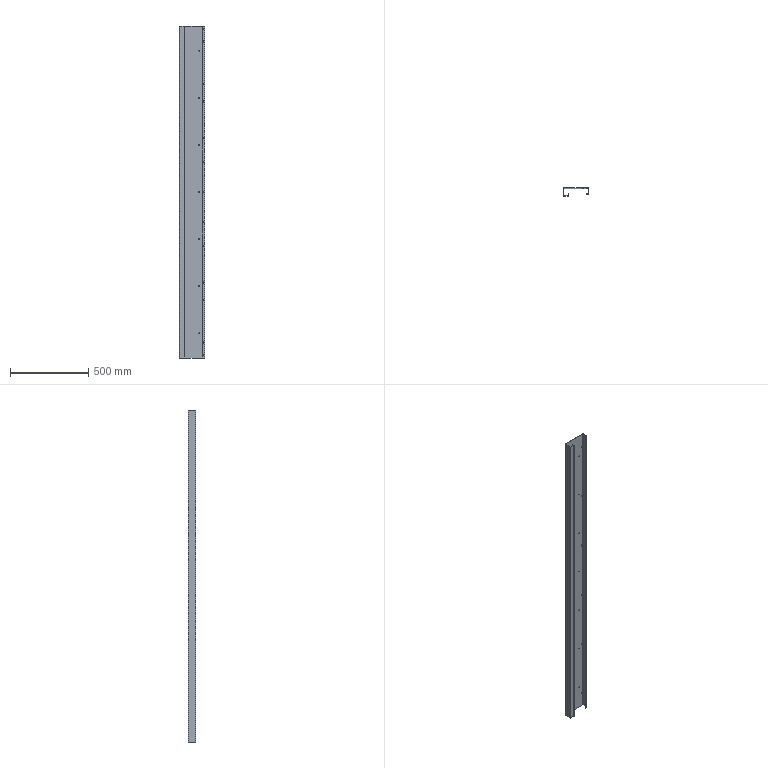Part | SolidWorks | features ICE 7, EdgeFlange 2, Cut 1, FlatPattern 1, SMBaseFlange 1, SheetMetal 1 | 1 solid | 130 faces | box 160.5 x 50 x 2116 mm | volume 758867 mm3 | cylinder 76 | plane 54 | commonest cylinder face diameters 6.2 x28 4.2 x14 8 x12 11 x12 1 x5 3.4 x5